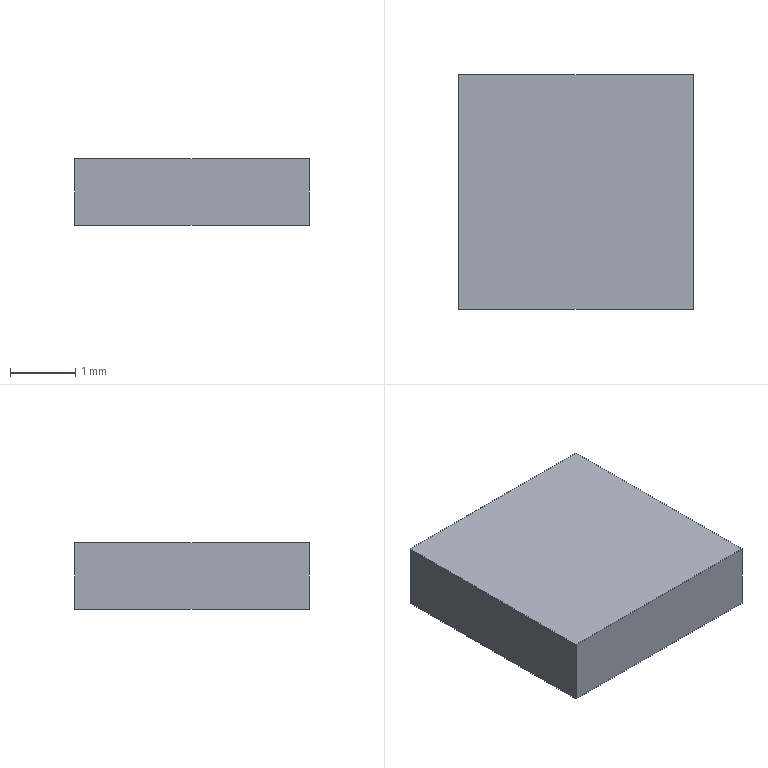Part | Creo | 1 solid | 6 faces | box 3.6 x 3.6 x 1.02 mm | volume 13.22 mm3 | plane 6
STEP:
#1=CARTESIAN_POINT('',(0.,0.,0.));
#2=DIRECTION('',(0.,0.,1.));
#3=DIRECTION('',(1.,0.,0.));
#4=AXIS2_PLACEMENT_3D('',#1,#2,#3);
#5=CARTESIAN_POINT('',(-1.8,1.8,0.));
#6=VERTEX_POINT('',#5);
#7=CARTESIAN_POINT('',(-1.8,-1.8,0.));
#8=VERTEX_POINT('',#7);
#9=CARTESIAN_POINT('',(-1.8,1.8,0.));
#10=DIRECTION('',(0.,-1.,0.));
#11=VECTOR('',#10,3.6);
#12=LINE('',#9,#11);
#13=EDGE_CURVE('',#6,#8,#12,.T.);
#14=ORIENTED_EDGE('',*,*,#13,.T.);
#15=CARTESIAN_POINT('',(1.8,-1.8,0.));
#16=VERTEX_POINT('',#15);
#17=CARTESIAN_POINT('',(-1.8,-1.8,0.));
#18=DIRECTION('',(1.,0.,0.));
#19=VECTOR('',#18,3.6);
#20=LINE('',#17,#19);
#21=EDGE_CURVE('',#8,#16,#20,.T.);
#22=ORIENTED_EDGE('',*,*,#21,.T.);
#23=CARTESIAN_POINT('',(1.8,1.8,0.));
#24=VERTEX_POINT('',#23);
#25=CARTESIAN_POINT('',(1.8,-1.8,0.));
#26=DIRECTION('',(0.,1.,0.));
#27=VECTOR('',#26,3.6);
#28=LINE('',#25,#27);
#29=EDGE_CURVE('',#16,#24,#28,.T.);
#30=ORIENTED_EDGE('',*,*,#29,.T.);
#31=CARTESIAN_POINT('',(1.8,1.8,0.));
#32=DIRECTION('',(-1.,0.,0.));
#33=VECTOR('',#32,3.6);
#34=LINE('',#31,#33);
#35=EDGE_CURVE('',#24,#6,#34,.T.);
#36=ORIENTED_EDGE('',*,*,#35,.T.);
#37=EDGE_LOOP('',(#14,#22,#30,#36));
#38=FACE_OUTER_BOUND('',#37,.F.);
#39=CARTESIAN_POINT('',(0.,0.,0.));
#40=DIRECTION('',(0.,0.,1.));
#41=DIRECTION('',(1.,0.,0.));
#42=AXIS2_PLACEMENT_3D('',#39,#40,#41);
#43=PLANE('',#42);
#44=ADVANCED_FACE('',(#38),#43,.F.);
#45=ORIENTED_EDGE('',*,*,#13,.F.);
#46=CARTESIAN_POINT('',(-1.8,1.8,1.02));
#47=VERTEX_POINT('',#46);
#48=CARTESIAN_POINT('',(-1.8,1.8,0.));
#49=DIRECTION('',(0.,0.,1.));
#50=VECTOR('',#49,1.02);
#51=LINE('',#48,#50);
#52=EDGE_CURVE('',#6,#47,#51,.T.);
#53=ORIENTED_EDGE('',*,*,#52,.T.);
#54=CARTESIAN_POINT('',(-1.8,-1.8,1.02));
#55=VERTEX_POINT('',#54);
#56=CARTESIAN_POINT('',(-1.8,1.8,1.02));
#57=DIRECTION('',(0.,-1.,0.));
#58=VECTOR('',#57,3.6);
#59=LINE('',#56,#58);
#60=EDGE_CURVE('',#47,#55,#59,.T.);
#61=ORIENTED_EDGE('',*,*,#60,.T.);
#62=CARTESIAN_POINT('',(-1.8,-1.8,0.));
#63=DIRECTION('',(0.,0.,1.));
#64=VECTOR('',#63,1.02);
#65=LINE('',#62,#64);
#66=EDGE_CURVE('',#8,#55,#65,.T.);
#67=ORIENTED_EDGE('',*,*,#66,.F.);
#68=EDGE_LOOP('',(#45,#53,#61,#67));
#69=FACE_OUTER_BOUND('',#68,.F.);
#70=CARTESIAN_POINT('',(-1.8,1.8,0.));
#71=DIRECTION('',(-1.,0.,0.));
#72=DIRECTION('',(0.,-1.,0.));
#73=AXIS2_PLACEMENT_3D('',#70,#71,#72);
#74=PLANE('',#73);
#75=ADVANCED_FACE('',(#69),#74,.T.);
#76=ORIENTED_EDGE('',*,*,#35,.F.);
#77=CARTESIAN_POINT('',(1.8,1.8,1.02));
#78=VERTEX_POINT('',#77);
#79=CARTESIAN_POINT('',(1.8,1.8,0.));
#80=DIRECTION('',(0.,0.,1.));
#81=VECTOR('',#80,1.02);
#82=LINE('',#79,#81);
#83=EDGE_CURVE('',#24,#78,#82,.T.);
#84=ORIENTED_EDGE('',*,*,#83,.T.);
#85=CARTESIAN_POINT('',(1.8,1.8,1.02));
#86=DIRECTION('',(-1.,0.,0.));
#87=VECTOR('',#86,3.6);
#88=LINE('',#85,#87);
#89=EDGE_CURVE('',#78,#47,#88,.T.);
#90=ORIENTED_EDGE('',*,*,#89,.T.);
#91=ORIENTED_EDGE('',*,*,#52,.F.);
#92=EDGE_LOOP('',(#76,#84,#90,#91));
#93=FACE_OUTER_BOUND('',#92,.F.);
#94=CARTESIAN_POINT('',(1.8,1.8,0.));
#95=DIRECTION('',(0.,1.,0.));
#96=DIRECTION('',(-1.,0.,0.));
#97=AXIS2_PLACEMENT_3D('',#94,#95,#96);
#98=PLANE('',#97);
#99=ADVANCED_FACE('',(#93),#98,.T.);
#100=ORIENTED_EDGE('',*,*,#29,.F.);
#101=CARTESIAN_POINT('',(1.8,-1.8,1.02));
#102=VERTEX_POINT('',#101);
#103=CARTESIAN_POINT('',(1.8,-1.8,0.));
#104=DIRECTION('',(0.,0.,1.));
#105=VECTOR('',#104,1.02);
#106=LINE('',#103,#105);
#107=EDGE_CURVE('',#16,#102,#106,.T.);
#108=ORIENTED_EDGE('',*,*,#107,.T.);
#109=CARTESIAN_POINT('',(1.8,-1.8,1.02));
#110=DIRECTION('',(0.,1.,0.));
#111=VECTOR('',#110,3.6);
#112=LINE('',#109,#111);
#113=EDGE_CURVE('',#102,#78,#112,.T.);
#114=ORIENTED_EDGE('',*,*,#113,.T.);
#115=ORIENTED_EDGE('',*,*,#83,.F.);
#116=EDGE_LOOP('',(#100,#108,#114,#115));
#117=FACE_OUTER_BOUND('',#116,.F.);
#118=CARTESIAN_POINT('',(1.8,-1.8,0.));
#119=DIRECTION('',(1.,0.,0.));
#120=DIRECTION('',(0.,1.,0.));
#121=AXIS2_PLACEMENT_3D('',#118,#119,#120);
#122=PLANE('',#121);
#123=ADVANCED_FACE('',(#117),#122,.T.);
#124=ORIENTED_EDGE('',*,*,#21,.F.);
#125=ORIENTED_EDGE('',*,*,#66,.T.);
#126=CARTESIAN_POINT('',(-1.8,-1.8,1.02));
#127=DIRECTION('',(1.,0.,0.));
#128=VECTOR('',#127,3.6);
#129=LINE('',#126,#128);
#130=EDGE_CURVE('',#55,#102,#129,.T.);
#131=ORIENTED_EDGE('',*,*,#130,.T.);
#132=ORIENTED_EDGE('',*,*,#107,.F.);
#133=EDGE_LOOP('',(#124,#125,#131,#132));
#134=FACE_OUTER_BOUND('',#133,.F.);
#135=CARTESIAN_POINT('',(-1.8,-1.8,0.));
#136=DIRECTION('',(0.,-1.,0.));
#137=DIRECTION('',(1.,0.,0.));
#138=AXIS2_PLACEMENT_3D('',#135,#136,#137);
#139=PLANE('',#138);
#140=ADVANCED_FACE('',(#134),#139,.T.);
#141=ORIENTED_EDGE('',*,*,#60,.F.);
#142=ORIENTED_EDGE('',*,*,#89,.F.);
#143=ORIENTED_EDGE('',*,*,#113,.F.);
#144=ORIENTED_EDGE('',*,*,#130,.F.);
#145=EDGE_LOOP('',(#141,#142,#143,#144));
#146=FACE_OUTER_BOUND('',#145,.F.);
#147=CARTESIAN_POINT('',(0.,0.,1.02));
#148=DIRECTION('',(0.,0.,1.));
#149=DIRECTION('',(1.,0.,0.));
#150=AXIS2_PLACEMENT_3D('',#147,#148,#149);
#151=PLANE('',#150);
#152=ADVANCED_FACE('',(#146),#151,.T.);
#153=CLOSED_SHELL('',(#44,#75,#99,#123,#140,#152));
#154=MANIFOLD_SOLID_BREP('',#153);
#155=(LENGTH_UNIT()NAMED_UNIT(*)SI_UNIT(.MILLI.,.METRE.));
#156=UNCERTAINTY_MEASURE_WITH_UNIT(LENGTH_MEASURE(0.0005192),#155,'','');
#157=(NAMED_UNIT(*)PLANE_ANGLE_UNIT()SI_UNIT($,.RADIAN.));
#158=PLANE_ANGLE_MEASURE_WITH_UNIT(PLANE_ANGLE_MEASURE(0.01745),#157);
#159=(CONVERSION_BASED_UNIT('DEGREE',#158)NAMED_UNIT(*)PLANE_ANGLE_UNIT());
#160=(NAMED_UNIT(*)SI_UNIT($,.STERADIAN.)SOLID_ANGLE_UNIT());
#161=(GEOMETRIC_REPRESENTATION_CONTEXT(3)GLOBAL_UNCERTAINTY_ASSIGNED_CONTEXT((#156))GLOBAL_UNIT_ASSIGNED_CONTEXT((#155,#159,#160))REPRESENTATION_CONTEXT('',''));
#162=ADVANCED_BREP_SHAPE_REPRESENTATION('',(#4,#154),#161);